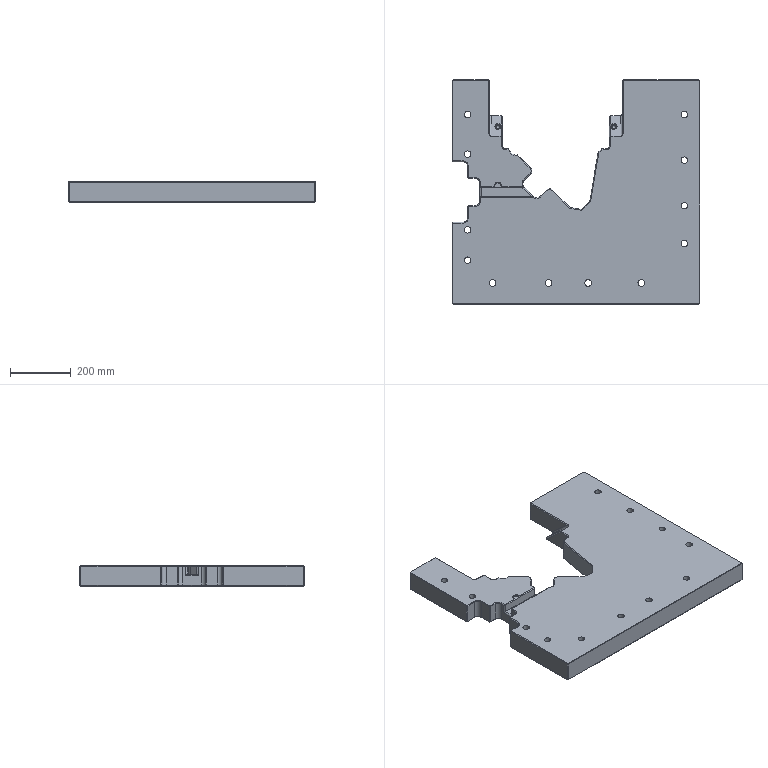Part | Creo | 1 solid | 252 faces | box 815 x 740 x 68.2 mm | volume 30758006 mm3 | plane 134 | cone 58 | cylinder 55 | spline 4 | torus 1 | commonest cylinder face diameters 21.5 x24 30 x8 10 x6 20 x5 10.579 x4 13 x4